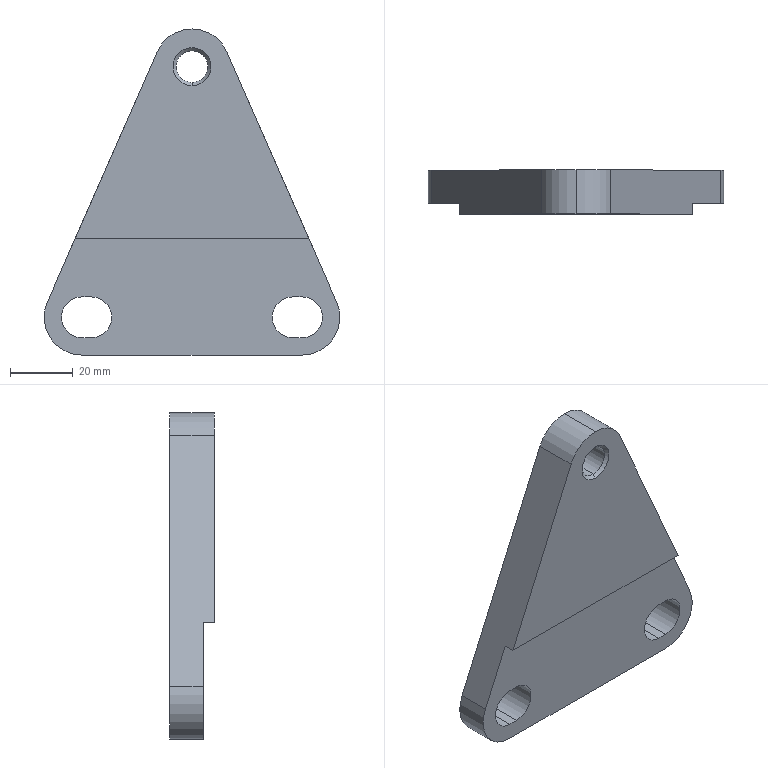Part | SolidWorks | features BaseBody 1 | 1 solid | 25 faces | box 94 x 14 x 103.649 mm | volume 70414 mm3 | plane 11 | cylinder 10 | cone 4 | commonest cylinder face diameters 13 x4 24 x4 10.106 x2
STEP:
#1=CARTESIAN_POINT('',(0.,-13.,96.702));
#2=VERTEX_POINT('',#1);
#3=CARTESIAN_POINT('',(0.,-13.,86.596));
#4=VERTEX_POINT('',#3);
#5=CARTESIAN_POINT('',(0.,-13.,91.649));
#6=DIRECTION('',(0.,-1.,0.));
#7=DIRECTION('',(0.,0.,-1.));
#8=AXIS2_PLACEMENT_3D('',#5,#6,#7);
#9=CIRCLE('',#8,5.053);
#10=EDGE_CURVE('',#2,#4,#9,.T.);
#11=ORIENTED_EDGE('',*,*,#10,.F.);
#12=CARTESIAN_POINT('',(0.,-14.,97.702));
#13=VERTEX_POINT('',#12);
#14=CARTESIAN_POINT('',(0.,-13.,96.702));
#15=DIRECTION('',(0.,-0.7071,0.7071));
#16=VECTOR('',#15,1000.);
#17=LINE('',#14,#16);
#18=EDGE_CURVE('',#2,#13,#17,.T.);
#19=ORIENTED_EDGE('',*,*,#18,.T.);
#20=CARTESIAN_POINT('',(0.,-14.,85.596));
#21=VERTEX_POINT('',#20);
#22=CARTESIAN_POINT('',(0.,-14.,91.649));
#23=DIRECTION('',(0.,1.,0.));
#24=DIRECTION('',(0.,0.,-1.));
#25=AXIS2_PLACEMENT_3D('',#22,#23,#24);
#26=CIRCLE('',#25,6.053);
#27=EDGE_CURVE('',#21,#13,#26,.T.);
#28=ORIENTED_EDGE('',*,*,#27,.F.);
#29=CARTESIAN_POINT('',(0.,-13.,86.596));
#30=DIRECTION('',(0.,-0.7071,-0.7071));
#31=VECTOR('',#30,1000.);
#32=LINE('',#29,#31);
#33=EDGE_CURVE('',#4,#21,#32,.T.);
#34=ORIENTED_EDGE('',*,*,#33,.F.);
#35=EDGE_LOOP('',(#11,#19,#28,#34));
#36=FACE_OUTER_BOUND('',#35,.T.);
#37=CARTESIAN_POINT('',(0.,-13.,91.649));
#38=DIRECTION('',(0.,-1.,0.));
#39=DIRECTION('',(0.,0.,-1.));
#40=AXIS2_PLACEMENT_3D('',#37,#38,#39);
#41=CONICAL_SURFACE('',#40,5.053,0.7854);
#42=ADVANCED_FACE('',(#36),#41,.F.);
#43=CARTESIAN_POINT('',(10.986,0.,96.477));
#44=VERTEX_POINT('',#43);
#45=CARTESIAN_POINT('',(0.,0.,103.649));
#46=VERTEX_POINT('',#45);
#47=CARTESIAN_POINT('',(0.,0.,91.649));
#48=DIRECTION('',(0.,-1.,0.));
#49=DIRECTION('',(1.,0.,0.));
#50=AXIS2_PLACEMENT_3D('',#47,#48,#49);
#51=CIRCLE('',#50,12.);
#52=EDGE_CURVE('',#44,#46,#51,.T.);
#53=ORIENTED_EDGE('',*,*,#52,.T.);
#54=CARTESIAN_POINT('',(0.,-14.,103.649));
#55=VERTEX_POINT('',#54);
#56=CARTESIAN_POINT('',(0.,-14.,103.649));
#57=DIRECTION('',(0.,-1.,0.));
#58=VECTOR('',#57,1000.);
#59=LINE('',#56,#58);
#60=EDGE_CURVE('',#46,#55,#59,.T.);
#61=ORIENTED_EDGE('',*,*,#60,.T.);
#62=CARTESIAN_POINT('',(10.986,-14.,96.477));
#63=VERTEX_POINT('',#62);
#64=CARTESIAN_POINT('',(0.,-14.,91.649));
#65=DIRECTION('',(0.,-1.,0.));
#66=DIRECTION('',(1.,0.,0.));
#67=AXIS2_PLACEMENT_3D('',#64,#65,#66);
#68=CIRCLE('',#67,12.);
#69=EDGE_CURVE('',#63,#55,#68,.T.);
#70=ORIENTED_EDGE('',*,*,#69,.F.);
#71=CARTESIAN_POINT('',(10.986,-14.,96.477));
#72=DIRECTION('',(0.,1.,0.));
#73=VECTOR('',#72,1000.);
#74=LINE('',#71,#73);
#75=EDGE_CURVE('',#63,#44,#74,.T.);
#76=ORIENTED_EDGE('',*,*,#75,.T.);
#77=EDGE_LOOP('',(#53,#61,#70,#76));
#78=FACE_OUTER_BOUND('',#77,.T.);
#79=CARTESIAN_POINT('',(0.,-14.,91.649));
#80=DIRECTION('',(0.,-1.,0.));
#81=DIRECTION('',(0.,0.,1.));
#82=AXIS2_PLACEMENT_3D('',#79,#80,#81);
#83=CYLINDRICAL_SURFACE('',#82,12.);
#84=ADVANCED_FACE('',(#78),#83,.T.);
#85=CARTESIAN_POINT('',(0.,-1.,86.596));
#86=VERTEX_POINT('',#85);
#87=CARTESIAN_POINT('',(0.,-1.,96.702));
#88=VERTEX_POINT('',#87);
#89=CARTESIAN_POINT('',(0.,-1.,91.649));
#90=DIRECTION('',(0.,1.,0.));
#91=DIRECTION('',(0.,0.,-1.));
#92=AXIS2_PLACEMENT_3D('',#89,#90,#91);
#93=CIRCLE('',#92,5.053);
#94=EDGE_CURVE('',#86,#88,#93,.T.);
#95=ORIENTED_EDGE('',*,*,#94,.F.);
#96=CARTESIAN_POINT('',(0.,0.,85.596));
#97=VERTEX_POINT('',#96);
#98=CARTESIAN_POINT('',(0.,0.,85.596));
#99=DIRECTION('',(0.,0.7071,-0.7071));
#100=VECTOR('',#99,1000.);
#101=LINE('',#98,#100);
#102=EDGE_CURVE('',#86,#97,#101,.T.);
#103=ORIENTED_EDGE('',*,*,#102,.T.);
#104=CARTESIAN_POINT('',(0.,0.,97.702));
#105=VERTEX_POINT('',#104);
#106=CARTESIAN_POINT('',(0.,0.,91.649));
#107=DIRECTION('',(0.,-1.,0.));
#108=DIRECTION('',(0.,0.,-1.));
#109=AXIS2_PLACEMENT_3D('',#106,#107,#108);
#110=CIRCLE('',#109,6.053);
#111=EDGE_CURVE('',#105,#97,#110,.T.);
#112=ORIENTED_EDGE('',*,*,#111,.F.);
#113=CARTESIAN_POINT('',(0.,0.,97.702));
#114=DIRECTION('',(0.,0.7071,0.7071));
#115=VECTOR('',#114,1000.);
#116=LINE('',#113,#115);
#117=EDGE_CURVE('',#88,#105,#116,.T.);
#118=ORIENTED_EDGE('',*,*,#117,.F.);
#119=EDGE_LOOP('',(#95,#103,#112,#118));
#120=FACE_OUTER_BOUND('',#119,.T.);
#121=CARTESIAN_POINT('',(0.,0.,91.649));
#122=DIRECTION('',(0.,1.,0.));
#123=DIRECTION('',(0.,0.,1.));
#124=AXIS2_PLACEMENT_3D('',#121,#122,#123);
#125=CONICAL_SURFACE('',#124,6.053,0.7854);
#126=ADVANCED_FACE('',(#120),#125,.F.);
#127=ORIENTED_EDGE('',*,*,#10,.T.);
#128=CARTESIAN_POINT('',(0.,-14.,86.596));
#129=DIRECTION('',(0.,1.,0.));
#130=VECTOR('',#129,1000.);
#131=LINE('',#128,#130);
#132=EDGE_CURVE('',#4,#86,#131,.T.);
#133=ORIENTED_EDGE('',*,*,#132,.T.);
#134=ORIENTED_EDGE('',*,*,#94,.T.);
#135=CARTESIAN_POINT('',(0.,-14.,96.702));
#136=DIRECTION('',(0.,1.,0.));
#137=VECTOR('',#136,1000.);
#138=LINE('',#135,#137);
#139=EDGE_CURVE('',#2,#88,#138,.T.);
#140=ORIENTED_EDGE('',*,*,#139,.F.);
#141=EDGE_LOOP('',(#127,#133,#134,#140));
#142=FACE_OUTER_BOUND('',#141,.T.);
#143=CARTESIAN_POINT('',(0.,-14.,91.649));
#144=DIRECTION('',(0.,1.,0.));
#145=DIRECTION('',(0.,0.,1.));
#146=AXIS2_PLACEMENT_3D('',#143,#144,#145);
#147=CYLINDRICAL_SURFACE('',#146,5.053);
#148=ADVANCED_FACE('',(#142),#147,.F.);
#149=CARTESIAN_POINT('',(-35.,0.,5.5));
#150=VERTEX_POINT('',#149);
#151=CARTESIAN_POINT('',(-35.,-10.5,5.5));
#152=VERTEX_POINT('',#151);
#153=CARTESIAN_POINT('',(-35.,0.,5.5));
#154=DIRECTION('',(0.,-1.,0.));
#155=VECTOR('',#154,1000.);
#156=LINE('',#153,#155);
#157=EDGE_CURVE('',#150,#152,#156,.T.);
#158=ORIENTED_EDGE('',*,*,#157,.T.);
#159=CARTESIAN_POINT('',(-32.,-10.5,5.5));
#160=VERTEX_POINT('',#159);
#161=CARTESIAN_POINT('',(-35.,-10.5,5.5));
#162=DIRECTION('',(1.,0.,0.));
#163=VECTOR('',#162,1000.);
#164=LINE('',#161,#163);
#165=EDGE_CURVE('',#152,#160,#164,.T.);
#166=ORIENTED_EDGE('',*,*,#165,.T.);
#167=CARTESIAN_POINT('',(-32.,0.,5.5));
#168=VERTEX_POINT('',#167);
#169=CARTESIAN_POINT('',(-32.,0.,5.5));
#170=DIRECTION('',(0.,-1.,0.));
#171=VECTOR('',#170,1000.);
#172=LINE('',#169,#171);
#173=EDGE_CURVE('',#168,#160,#172,.T.);
#174=ORIENTED_EDGE('',*,*,#173,.F.);
#175=CARTESIAN_POINT('',(-35.,0.,5.5));
#176=DIRECTION('',(-1.,0.,0.));
#177=VECTOR('',#176,1000.);
#178=LINE('',#175,#177);
#179=EDGE_CURVE('',#168,#150,#178,.T.);
#180=ORIENTED_EDGE('',*,*,#179,.T.);
#181=EDGE_LOOP('',(#158,#166,#174,#180));
#182=FACE_OUTER_BOUND('',#181,.T.);
#183=CARTESIAN_POINT('',(-35.,0.,5.5));
#184=DIRECTION('',(0.,0.,1.));
#185=DIRECTION('',(1.,0.,0.));
#186=AXIS2_PLACEMENT_3D('',#183,#184,#185);
#187=PLANE('',#186);
#188=ADVANCED_FACE('',(#182),#187,.T.);
#189=ORIENTED_EDGE('',*,*,#132,.F.);
#190=CARTESIAN_POINT('',(0.,-13.,91.649));
#191=DIRECTION('',(0.,-1.,0.));
#192=DIRECTION('',(0.,0.,-1.));
#193=AXIS2_PLACEMENT_3D('',#190,#191,#192);
#194=CIRCLE('',#193,5.053);
#195=EDGE_CURVE('',#4,#2,#194,.T.);
#196=ORIENTED_EDGE('',*,*,#195,.T.);
#197=ORIENTED_EDGE('',*,*,#139,.T.);
#198=CARTESIAN_POINT('',(0.,-1.,91.649));
#199=DIRECTION('',(0.,1.,0.));
#200=DIRECTION('',(0.,0.,-1.));
#201=AXIS2_PLACEMENT_3D('',#198,#199,#200);
#202=CIRCLE('',#201,5.053);
#203=EDGE_CURVE('',#88,#86,#202,.T.);
#204=ORIENTED_EDGE('',*,*,#203,.T.);
#205=EDGE_LOOP('',(#189,#196,#197,#204));
#206=FACE_OUTER_BOUND('',#205,.T.);
#207=CARTESIAN_POINT('',(0.,-14.,91.649));
#208=DIRECTION('',(0.,1.,0.));
#209=DIRECTION('',(0.,0.,1.));
#210=AXIS2_PLACEMENT_3D('',#207,#208,#209);
#211=CYLINDRICAL_SURFACE('',#210,5.053);
#212=ADVANCED_FACE('',(#206),#211,.F.);
#213=ORIENTED_EDGE('',*,*,#102,.F.);
#214=ORIENTED_EDGE('',*,*,#203,.F.);
#215=ORIENTED_EDGE('',*,*,#117,.T.);
#216=CARTESIAN_POINT('',(0.,0.,91.649));
#217=DIRECTION('',(0.,-1.,0.));
#218=DIRECTION('',(0.,0.,-1.));
#219=AXIS2_PLACEMENT_3D('',#216,#217,#218);
#220=CIRCLE('',#219,6.053);
#221=EDGE_CURVE('',#97,#105,#220,.T.);
#222=ORIENTED_EDGE('',*,*,#221,.F.);
#223=EDGE_LOOP('',(#213,#214,#215,#222));
#224=FACE_OUTER_BOUND('',#223,.T.);
#225=CARTESIAN_POINT('',(0.,0.,91.649));
#226=DIRECTION('',(0.,1.,0.));
#227=DIRECTION('',(0.,0.,1.));
#228=AXIS2_PLACEMENT_3D('',#225,#226,#227);
#229=CONICAL_SURFACE('',#228,6.053,0.7854);
#230=ADVANCED_FACE('',(#224),#229,.F.);
#231=ORIENTED_EDGE('',*,*,#60,.F.);
#232=CARTESIAN_POINT('',(-10.986,0.,96.477));
#233=VERTEX_POINT('',#232);
#234=CARTESIAN_POINT('',(0.,0.,91.649));
#235=DIRECTION('',(0.,-1.,0.));
#236=DIRECTION('',(1.,0.,0.));
#237=AXIS2_PLACEMENT_3D('',#234,#235,#236);
#238=CIRCLE('',#237,12.);
#239=EDGE_CURVE('',#46,#233,#238,.T.);
#240=ORIENTED_EDGE('',*,*,#239,.T.);
#241=CARTESIAN_POINT('',(-10.986,-14.,96.477));
#242=VERTEX_POINT('',#241);
#243=CARTESIAN_POINT('',(-10.986,-14.,96.477));
#244=DIRECTION('',(0.,1.,0.));
#245=VECTOR('',#244,1000.);
#246=LINE('',#243,#245);
#247=EDGE_CURVE('',#242,#233,#246,.T.);
#248=ORIENTED_EDGE('',*,*,#247,.F.);
#249=CARTESIAN_POINT('',(0.,-14.,91.649));
#250=DIRECTION('',(0.,-1.,0.));
#251=DIRECTION('',(1.,0.,0.));
#252=AXIS2_PLACEMENT_3D('',#249,#250,#251);
#253=CIRCLE('',#252,12.);
#254=EDGE_CURVE('',#55,#242,#253,.T.);
#255=ORIENTED_EDGE('',*,*,#254,.F.);
#256=EDGE_LOOP('',(#231,#240,#248,#255));
#257=FACE_OUTER_BOUND('',#256,.T.);
#258=CARTESIAN_POINT('',(0.,-14.,91.649));
#259=DIRECTION('',(0.,-1.,0.));
#260=DIRECTION('',(0.,0.,1.));
#261=AXIS2_PLACEMENT_3D('',#258,#259,#260);
#262=CYLINDRICAL_SURFACE('',#261,12.);
#263=ADVANCED_FACE('',(#257),#262,.T.);
#264=CARTESIAN_POINT('',(35.,-10.5,0.));
#265=VERTEX_POINT('',#264);
#266=CARTESIAN_POINT('',(45.986,-10.5,16.828));
#267=VERTEX_POINT('',#266);
#268=CARTESIAN_POINT('',(35.,-10.5,12.));
#269=DIRECTION('',(0.,-1.,0.));
#270=DIRECTION('',(0.,0.,-1.));
#271=AXIS2_PLACEMENT_3D('',#268,#269,#270);
#272=CIRCLE('',#271,12.);
#273=EDGE_CURVE('',#265,#267,#272,.T.);
#274=ORIENTED_EDGE('',*,*,#273,.F.);
#275=CARTESIAN_POINT('',(35.,0.,0.));
#276=VERTEX_POINT('',#275);
#277=CARTESIAN_POINT('',(35.,-14.,0.));
#278=DIRECTION('',(0.,1.,0.));
#279=VECTOR('',#278,1000.);
#280=LINE('',#277,#279);
#281=EDGE_CURVE('',#265,#276,#280,.T.);
#282=ORIENTED_EDGE('',*,*,#281,.T.);
#283=CARTESIAN_POINT('',(45.986,0.,16.828));
#284=VERTEX_POINT('',#283);
#285=CARTESIAN_POINT('',(35.,0.,12.));
#286=DIRECTION('',(0.,-1.,0.));
#287=DIRECTION('',(-1.,0.,0.));
#288=AXIS2_PLACEMENT_3D('',#285,#286,#287);
#289=CIRCLE('',#288,12.);
#290=EDGE_CURVE('',#276,#284,#289,.T.);
#291=ORIENTED_EDGE('',*,*,#290,.T.);
#292=CARTESIAN_POINT('',(45.986,-14.,16.828));
#293=DIRECTION('',(0.,1.,0.));
#294=VECTOR('',#293,1000.);
#295=LINE('',#292,#294);
#296=EDGE_CURVE('',#267,#284,#295,.T.);
#297=ORIENTED_EDGE('',*,*,#296,.F.);
#298=EDGE_LOOP('',(#274,#282,#291,#297));
#299=FACE_OUTER_BOUND('',#298,.T.);
#300=CARTESIAN_POINT('',(35.,-14.,12.));
#301=DIRECTION('',(0.,-1.,0.));
#302=DIRECTION('',(0.,0.,1.));
#303=AXIS2_PLACEMENT_3D('',#300,#301,#302);
#304=CYLINDRICAL_SURFACE('',#303,12.);
#305=ADVANCED_FACE('',(#299),#304,.T.);
#306=CARTESIAN_POINT('',(-35.,-10.5,0.));
#307=VERTEX_POINT('',#306);
#308=CARTESIAN_POINT('',(-50.,-10.5,0.));
#309=DIRECTION('',(1.,0.,0.));
#310=VECTOR('',#309,1000.);
#311=LINE('',#308,#310);
#312=EDGE_CURVE('',#307,#265,#311,.T.);
#313=ORIENTED_EDGE('',*,*,#312,.F.);
#314=CARTESIAN_POINT('',(-35.,0.,0.));
#315=VERTEX_POINT('',#314);
#316=CARTESIAN_POINT('',(-35.,-14.,0.));
#317=DIRECTION('',(0.,1.,0.));
#318=VECTOR('',#317,1000.);
#319=LINE('',#316,#318);
#320=EDGE_CURVE('',#307,#315,#319,.T.);
#321=ORIENTED_EDGE('',*,*,#320,.T.);
#322=CARTESIAN_POINT('',(-35.,0.,0.));
#323=DIRECTION('',(1.,0.,0.));
#324=VECTOR('',#323,1000.);
#325=LINE('',#322,#324);
#326=EDGE_CURVE('',#315,#276,#325,.T.);
#327=ORIENTED_EDGE('',*,*,#326,.T.);
#328=ORIENTED_EDGE('',*,*,#281,.F.);
#329=EDGE_LOOP('',(#313,#321,#327,#328));
#330=FACE_OUTER_BOUND('',#329,.T.);
#331=CARTESIAN_POINT('',(-35.,-14.,0.));
#332=DIRECTION('',(0.,0.,1.));
#333=DIRECTION('',(1.,0.,0.));
#334=AXIS2_PLACEMENT_3D('',#331,#332,#333);
#335=PLANE('',#334);
#336=ADVANCED_FACE('',(#330),#335,.F.);
#337=CARTESIAN_POINT('',(-37.122,-10.5,37.));
#338=VERTEX_POINT('',#337);
#339=CARTESIAN_POINT('',(-45.986,-10.5,16.828));
#340=VERTEX_POINT('',#339);
#341=CARTESIAN_POINT('',(-10.986,-10.5,96.477));
#342=DIRECTION('',(-0.4023,0.,-0.9155));
#343=VECTOR('',#342,1000.);
#344=LINE('',#341,#343);
#345=EDGE_CURVE('',#338,#340,#344,.T.);
#346=ORIENTED_EDGE('',*,*,#345,.F.);
#347=CARTESIAN_POINT('',(-37.122,-14.,37.));
#348=VERTEX_POINT('',#347);
#349=CARTESIAN_POINT('',(-37.122,-14.,37.));
#350=DIRECTION('',(0.,-1.,0.));
#351=VECTOR('',#350,1000.);
#352=LINE('',#349,#351);
#353=EDGE_CURVE('',#338,#348,#352,.T.);
#354=ORIENTED_EDGE('',*,*,#353,.T.);
#355=CARTESIAN_POINT('',(-10.986,-14.,96.477));
#356=DIRECTION('',(-0.4023,0.,-0.9155));
#357=VECTOR('',#356,1000.);
#358=LINE('',#355,#357);
#359=EDGE_CURVE('',#242,#348,#358,.T.);
#360=ORIENTED_EDGE('',*,*,#359,.F.);
#361=ORIENTED_EDGE('',*,*,#247,.T.);
#362=CARTESIAN_POINT('',(-45.986,0.,16.828));
#363=VERTEX_POINT('',#362);
#364=CARTESIAN_POINT('',(-10.986,0.,96.477));
#365=DIRECTION('',(-0.4023,0.,-0.9155));
#366=VECTOR('',#365,1000.);
#367=LINE('',#364,#366);
#368=EDGE_CURVE('',#233,#363,#367,.T.);
#369=ORIENTED_EDGE('',*,*,#368,.T.);
#370=CARTESIAN_POINT('',(-45.986,-14.,16.828));
#371=DIRECTION('',(0.,1.,0.));
#372=VECTOR('',#371,1000.);
#373=LINE('',#370,#372);
#374=EDGE_CURVE('',#340,#363,#373,.T.);
#375=ORIENTED_EDGE('',*,*,#374,.F.);
#376=EDGE_LOOP('',(#346,#354,#360,#361,#369,#375));
#377=FACE_OUTER_BOUND('',#376,.T.);
#378=CARTESIAN_POINT('',(-10.986,-14.,96.477));
#379=DIRECTION('',(0.9155,0.,-0.4023));
#380=DIRECTION('',(0.,-1.,0.));
#381=AXIS2_PLACEMENT_3D('',#378,#379,#380);
#382=PLANE('',#381);
#383=ADVANCED_FACE('',(#377),#382,.F.);
#384=CARTESIAN_POINT('',(32.,-10.5,18.5));
#385=VERTEX_POINT('',#384);
#386=CARTESIAN_POINT('',(35.,-10.5,18.5));
#387=VERTEX_POINT('',#386);
#388=CARTESIAN_POINT('',(35.,-10.5,18.5));
#389=DIRECTION('',(1.,0.,0.));
#390=VECTOR('',#389,1000.);
#391=LINE('',#388,#390);
#392=EDGE_CURVE('',#385,#387,#391,.T.);
#393=ORIENTED_EDGE('',*,*,#392,.F.);
#394=CARTESIAN_POINT('',(32.,0.,18.5));
#395=VERTEX_POINT('',#394);
#396=CARTESIAN_POINT('',(32.,0.,18.5));
#397=DIRECTION('',(0.,-1.,0.));
#398=VECTOR('',#397,1000.);
#399=LINE('',#396,#398);
#400=EDGE_CURVE('',#395,#385,#399,.T.);
#401=ORIENTED_EDGE('',*,*,#400,.F.);
#402=CARTESIAN_POINT('',(35.,0.,18.5));
#403=VERTEX_POINT('',#402);
#404=CARTESIAN_POINT('',(35.,0.,18.5));
#405=DIRECTION('',(-1.,0.,0.));
#406=VECTOR('',#405,1000.);
#407=LINE('',#404,#406);
#408=EDGE_CURVE('',#403,#395,#407,.T.);
#409=ORIENTED_EDGE('',*,*,#408,.F.);
#410=CARTESIAN_POINT('',(35.,0.,18.5));
#411=DIRECTION('',(0.,-1.,0.));
#412=VECTOR('',#411,1000.);
#413=LINE('',#410,#412);
#414=EDGE_CURVE('',#403,#387,#413,.T.);
#415=ORIENTED_EDGE('',*,*,#414,.T.);
#416=EDGE_LOOP('',(#393,#401,#409,#415));
#417=FACE_OUTER_BOUND('',#416,.T.);
#418=CARTESIAN_POINT('',(35.,0.,18.5));
#419=DIRECTION('',(0.,0.,1.));
#420=DIRECTION('',(1.,0.,0.));
#421=AXIS2_PLACEMENT_3D('',#418,#419,#420);
#422=PLANE('',#421);
#423=ADVANCED_FACE('',(#417),#422,.F.);
#424=CARTESIAN_POINT('',(35.,-10.5,5.5));
#425=VERTEX_POINT('',#424);
#426=CARTESIAN_POINT('',(35.,-10.5,12.));
#427=DIRECTION('',(0.,1.,0.));
#428=DIRECTION('',(0.,0.,-1.));
#429=AXIS2_PLACEMENT_3D('',#426,#427,#428);
#430=CIRCLE('',#429,6.5);
#431=EDGE_CURVE('',#387,#425,#430,.T.);
#432=ORIENTED_EDGE('',*,*,#431,.F.);
#433=ORIENTED_EDGE('',*,*,#414,.F.);
#434=CARTESIAN_POINT('',(35.,0.,5.5));
#435=VERTEX_POINT('',#434);
#436=CARTESIAN_POINT('',(35.,0.,12.));
#437=DIRECTION('',(0.,-1.,0.));
#438=DIRECTION('',(-1.,0.,0.));
#439=AXIS2_PLACEMENT_3D('',#436,#437,#438);
#440=CIRCLE('',#439,6.5);
#441=EDGE_CURVE('',#435,#403,#440,.T.);
#442=ORIENTED_EDGE('',*,*,#441,.F.);
#443=CARTESIAN_POINT('',(35.,0.,5.5));
#444=DIRECTION('',(0.,-1.,0.));
#445=VECTOR('',#444,1000.);
#446=LINE('',#443,#445);
#447=EDGE_CURVE('',#435,#425,#446,.T.);
#448=ORIENTED_EDGE('',*,*,#447,.T.);
#449=EDGE_LOOP('',(#432,#433,#442,#448));
#450=FACE_OUTER_BOUND('',#449,.T.);
#451=CARTESIAN_POINT('',(35.,0.,12.));
#452=DIRECTION('',(0.,1.,0.));
#453=DIRECTION('',(0.,0.,-1.));
#454=AXIS2_PLACEMENT_3D('',#451,#452,#453);
#455=CYLINDRICAL_SURFACE('',#454,6.5);
#456=ADVANCED_FACE('',(#450),#455,.F.);
#457=ORIENTED_EDGE('',*,*,#173,.T.);
#458=CARTESIAN_POINT('',(-32.,-10.5,18.5));
#459=VERTEX_POINT('',#458);
#460=CARTESIAN_POINT('',(-32.,-10.5,12.));
#461=DIRECTION('',(0.,-1.,0.));
#462=DIRECTION('',(0.,0.,-1.));
#463=AXIS2_PLACEMENT_3D('',#460,#461,#462);
#464=CIRCLE('',#463,6.5);
#465=EDGE_CURVE('',#160,#459,#464,.T.);
#466=ORIENTED_EDGE('',*,*,#465,.T.);
#467=CARTESIAN_POINT('',(-32.,0.,18.5));
#468=VERTEX_POINT('',#467);
#469=CARTESIAN_POINT('',(-32.,0.,18.5));
#470=DIRECTION('',(0.,-1.,0.));
#471=VECTOR('',#470,1000.);
#472=LINE('',#469,#471);
#473=EDGE_CURVE('',#468,#459,#472,.T.);
#474=ORIENTED_EDGE('',*,*,#473,.F.);
#475=CARTESIAN_POINT('',(-32.,0.,12.));
#476=DIRECTION('',(0.,1.,0.));
#477=DIRECTION('',(-1.,0.,0.));
#478=AXIS2_PLACEMENT_3D('',#475,#476,#477);
#479=CIRCLE('',#478,6.5);
#480=EDGE_CURVE('',#468,#168,#479,.T.);
#481=ORIENTED_EDGE('',*,*,#480,.T.);
#482=EDGE_LOOP('',(#457,#466,#474,#481));
#483=FACE_OUTER_BOUND('',#482,.T.);
#484=CARTESIAN_POINT('',(-32.,0.,12.));
#485=DIRECTION('',(0.,1.,0.));
#486=DIRECTION('',(0.,0.,-1.));
#487=AXIS2_PLACEMENT_3D('',#484,#485,#486);
#488=CYLINDRICAL_SURFACE('',#487,6.5);
#489=ADVANCED_FACE('',(#483),#488,.F.);
#490=CARTESIAN_POINT('',(-35.,0.,18.5));
#491=VERTEX_POINT('',#490);
#492=CARTESIAN_POINT('',(-35.,0.,12.));
#493=DIRECTION('',(0.,1.,0.));
#494=DIRECTION('',(1.,0.,0.));
#495=AXIS2_PLACEMENT_3D('',#492,#493,#494);
#496=CIRCLE('',#495,6.5);
#497=EDGE_CURVE('',#150,#491,#496,.T.);
#498=ORIENTED_EDGE('',*,*,#497,.F.);
#499=ORIENTED_EDGE('',*,*,#179,.F.);
#500=ORIENTED_EDGE('',*,*,#480,.F.);
#501=CARTESIAN_POINT('',(-35.,0.,18.5));
#502=DIRECTION('',(1.,0.,0.));
#503=VECTOR('',#502,1000.);
#504=LINE('',#501,#503);
#505=EDGE_CURVE('',#491,#468,#504,.T.);
#506=ORIENTED_EDGE('',*,*,#505,.F.);
#507=EDGE_LOOP('',(#498,#499,#500,#506));
#508=FACE_BOUND('',#507,.T.);
#509=ORIENTED_EDGE('',*,*,#52,.F.);
#510=CARTESIAN_POINT('',(45.986,0.,16.828));
#511=DIRECTION('',(-0.4023,0.,0.9155));
#512=VECTOR('',#511,1000.);
#513=LINE('',#510,#512);
#514=EDGE_CURVE('',#284,#44,#513,.T.);
#515=ORIENTED_EDGE('',*,*,#514,.F.);
#516=ORIENTED_EDGE('',*,*,#290,.F.);
#517=ORIENTED_EDGE('',*,*,#326,.F.);
#518=CARTESIAN_POINT('',(-35.,0.,12.));
#519=DIRECTION('',(0.,-1.,0.));
#520=DIRECTION('',(1.,0.,0.));
#521=AXIS2_PLACEMENT_3D('',#518,#519,#520);
#522=CIRCLE('',#521,12.);
#523=EDGE_CURVE('',#363,#315,#522,.T.);
#524=ORIENTED_EDGE('',*,*,#523,.F.);
#525=ORIENTED_EDGE('',*,*,#368,.F.);
#526=ORIENTED_EDGE('',*,*,#239,.F.);
#527=EDGE_LOOP('',(#509,#515,#516,#517,#524,#525,#526));
#528=FACE_OUTER_BOUND('',#527,.T.);
#529=CARTESIAN_POINT('',(32.,0.,5.5));
#530=VERTEX_POINT('',#529);
#531=CARTESIAN_POINT('',(35.,0.,5.5));
#532=DIRECTION('',(1.,0.,0.));
#533=VECTOR('',#532,1000.);
#534=LINE('',#531,#533);
#535=EDGE_CURVE('',#530,#435,#534,.T.);
#536=ORIENTED_EDGE('',*,*,#535,.T.);
#537=ORIENTED_EDGE('',*,*,#441,.T.);
#538=ORIENTED_EDGE('',*,*,#408,.T.);
#539=CARTESIAN_POINT('',(32.,0.,12.));
#540=DIRECTION('',(0.,-1.,0.));
#541=DIRECTION('',(1.,0.,0.));
#542=AXIS2_PLACEMENT_3D('',#539,#540,#541);
#543=CIRCLE('',#542,6.5);
#544=EDGE_CURVE('',#395,#530,#543,.T.);
#545=ORIENTED_EDGE('',*,*,#544,.T.);
#546=EDGE_LOOP('',(#536,#537,#538,#545));
#547=FACE_BOUND('',#546,.T.);
#548=ORIENTED_EDGE('',*,*,#111,.T.);
#549=ORIENTED_EDGE('',*,*,#221,.T.);
#550=EDGE_LOOP('',(#548,#549));
#551=FACE_BOUND('',#550,.T.);
#552=CARTESIAN_POINT('',(0.,0.,91.649));
#553=DIRECTION('',(0.,-1.,0.));
#554=DIRECTION('',(0.,0.,-1.));
#555=AXIS2_PLACEMENT_3D('',#552,#553,#554);
#556=PLANE('',#555);
#557=ADVANCED_FACE('',(#508,#528,#547,#551),#556,.F.);
#558=ORIENTED_EDGE('',*,*,#473,.T.);
#559=CARTESIAN_POINT('',(-35.,-10.5,18.5));
#560=VERTEX_POINT('',#559);
#561=CARTESIAN_POINT('',(-35.,-10.5,18.5));
#562=DIRECTION('',(-1.,0.,0.));
#563=VECTOR('',#562,1000.);
#564=LINE('',#561,#563);
#565=EDGE_CURVE('',#459,#560,#564,.T.);
#566=ORIENTED_EDGE('',*,*,#565,.T.);
#567=CARTESIAN_POINT('',(-35.,0.,18.5));
#568=DIRECTION('',(0.,-1.,0.));
#569=VECTOR('',#568,1000.);
#570=LINE('',#567,#569);
#571=EDGE_CURVE('',#491,#560,#570,.T.);
#572=ORIENTED_EDGE('',*,*,#571,.F.);
#573=ORIENTED_EDGE('',*,*,#505,.T.);
#574=EDGE_LOOP('',(#558,#566,#572,#573));
#575=FACE_OUTER_BOUND('',#574,.T.);
#576=CARTESIAN_POINT('',(-35.,0.,18.5));
#577=DIRECTION('',(0.,0.,-1.));
#578=DIRECTION('',(0.,-1.,0.));
#579=AXIS2_PLACEMENT_3D('',#576,#577,#578);
#580=PLANE('',#579);
#581=ADVANCED_FACE('',(#575),#580,.T.);
#582=ORIENTED_EDGE('',*,*,#571,.T.);
#583=CARTESIAN_POINT('',(-35.,-10.5,12.));
#584=DIRECTION('',(0.,-1.,0.));
#585=DIRECTION('',(0.,0.,-1.));
#586=AXIS2_PLACEMENT_3D('',#583,#584,#585);
#587=CIRCLE('',#586,6.5);
#588=EDGE_CURVE('',#560,#152,#587,.T.);
#589=ORIENTED_EDGE('',*,*,#588,.T.);
#590=ORIENTED_EDGE('',*,*,#157,.F.);
#591=ORIENTED_EDGE('',*,*,#497,.T.);
#592=EDGE_LOOP('',(#582,#589,#590,#591));
#593=FACE_OUTER_BOUND('',#592,.T.);
#594=CARTESIAN_POINT('',(-35.,0.,12.));
#595=DIRECTION('',(0.,1.,0.));
#596=DIRECTION('',(0.,0.,-1.));
#597=AXIS2_PLACEMENT_3D('',#594,#595,#596);
#598=CYLINDRICAL_SURFACE('',#597,6.5);
#599=ADVANCED_FACE('',(#593),#598,.F.);
#600=CARTESIAN_POINT('',(32.,-10.5,5.5));
#601=VERTEX_POINT('',#600);
#602=CARTESIAN_POINT('',(35.,-10.5,5.5));
#603=DIRECTION('',(-1.,0.,0.));
#604=VECTOR('',#603,1000.);
#605=LINE('',#602,#604);
#606=EDGE_CURVE('',#425,#601,#605,.T.);
#607=ORIENTED_EDGE('',*,*,#606,.F.);
#608=ORIENTED_EDGE('',*,*,#447,.F.);
#609=ORIENTED_EDGE('',*,*,#535,.F.);
#610=CARTESIAN_POINT('',(32.,0.,5.5));
#611=DIRECTION('',(0.,-1.,0.));
#612=VECTOR('',#611,1000.);
#613=LINE('',#610,#612);
#614=EDGE_CURVE('',#530,#601,#613,.T.);
#615=ORIENTED_EDGE('',*,*,#614,.T.);
#616=EDGE_LOOP('',(#607,#608,#609,#615));
#617=FACE_OUTER_BOUND('',#616,.T.);
#618=CARTESIAN_POINT('',(35.,0.,5.5));
#619=DIRECTION('',(0.,0.,-1.));
#620=DIRECTION('',(0.,-1.,0.));
#621=AXIS2_PLACEMENT_3D('',#618,#619,#620);
#622=PLANE('',#621);
#623=ADVANCED_FACE('',(#617),#622,.F.);
#624=CARTESIAN_POINT('',(32.,-10.5,12.));
#625=DIRECTION('',(0.,1.,0.));
#626=DIRECTION('',(0.,0.,-1.));
#627=AXIS2_PLACEMENT_3D('',#624,#625,#626);
#628=CIRCLE('',#627,6.5);
#629=EDGE_CURVE('',#601,#385,#628,.T.);
#630=ORIENTED_EDGE('',*,*,#629,.F.);
#631=ORIENTED_EDGE('',*,*,#614,.F.);
#632=ORIENTED_EDGE('',*,*,#544,.F.);
#633=ORIENTED_EDGE('',*,*,#400,.T.);
#634=EDGE_LOOP('',(#630,#631,#632,#633));
#635=FACE_OUTER_BOUND('',#634,.T.);
#636=CARTESIAN_POINT('',(32.,0.,12.));
#637=DIRECTION('',(0.,1.,0.));
#638=DIRECTION('',(0.,0.,-1.));
#639=AXIS2_PLACEMENT_3D('',#636,#637,#638);
#640=CYLINDRICAL_SURFACE('',#639,6.5);
#641=ADVANCED_FACE('',(#635),#640,.F.);
#642=ORIENTED_EDGE('',*,*,#345,.T.);
#643=CARTESIAN_POINT('',(-35.,-10.5,12.));
#644=DIRECTION('',(0.,-1.,0.));
#645=DIRECTION('',(0.,0.,-1.));
#646=AXIS2_PLACEMENT_3D('',#643,#644,#645);
#647=CIRCLE('',#646,12.);
#648=EDGE_CURVE('',#340,#307,#647,.T.);
#649=ORIENTED_EDGE('',*,*,#648,.T.);
#650=ORIENTED_EDGE('',*,*,#312,.T.);
#651=ORIENTED_EDGE('',*,*,#273,.T.);
#652=CARTESIAN_POINT('',(37.122,-10.5,37.));
#653=VERTEX_POINT('',#652);
#654=CARTESIAN_POINT('',(45.986,-10.5,16.828));
#655=DIRECTION('',(-0.4023,0.,0.9155));
#656=VECTOR('',#655,1000.);
#657=LINE('',#654,#656);
#658=EDGE_CURVE('',#267,#653,#657,.T.);
#659=ORIENTED_EDGE('',*,*,#658,.T.);
#660=CARTESIAN_POINT('',(50.,-10.5,37.));
#661=DIRECTION('',(-1.,0.,0.));
#662=VECTOR('',#661,1000.);
#663=LINE('',#660,#662);
#664=EDGE_CURVE('',#653,#338,#663,.T.);
#665=ORIENTED_EDGE('',*,*,#664,.T.);
#666=EDGE_LOOP('',(#642,#649,#650,#651,#659,#665));
#667=FACE_OUTER_BOUND('',#666,.T.);
#668=ORIENTED_EDGE('',*,*,#431,.T.);
#669=ORIENTED_EDGE('',*,*,#606,.T.);
#670=ORIENTED_EDGE('',*,*,#629,.T.);
#671=ORIENTED_EDGE('',*,*,#392,.T.);
#672=EDGE_LOOP('',(#668,#669,#670,#671));
#673=FACE_BOUND('',#672,.T.);
#674=ORIENTED_EDGE('',*,*,#565,.F.);
#675=ORIENTED_EDGE('',*,*,#465,.F.);
#676=ORIENTED_EDGE('',*,*,#165,.F.);
#677=ORIENTED_EDGE('',*,*,#588,.F.);
#678=EDGE_LOOP('',(#674,#675,#676,#677));
#679=FACE_BOUND('',#678,.T.);
#680=CARTESIAN_POINT('',(50.,-10.5,0.));
#681=DIRECTION('',(0.,-1.,0.));
#682=DIRECTION('',(0.,0.,-1.));
#683=AXIS2_PLACEMENT_3D('',#680,#681,#682);
#684=PLANE('',#683);
#685=ADVANCED_FACE('',(#667,#673,#679),#684,.T.);
#686=CARTESIAN_POINT('',(37.122,-14.,37.));
#687=VERTEX_POINT('',#686);
#688=CARTESIAN_POINT('',(45.986,-14.,16.828));
#689=DIRECTION('',(-0.4023,0.,0.9155));
#690=VECTOR('',#689,1000.);
#691=LINE('',#688,#690);
#692=EDGE_CURVE('',#687,#63,#691,.T.);
#693=ORIENTED_EDGE('',*,*,#692,.F.);
#694=CARTESIAN_POINT('',(37.122,-14.,37.));
#695=DIRECTION('',(0.,1.,0.));
#696=VECTOR('',#695,1000.);
#697=LINE('',#694,#696);
#698=EDGE_CURVE('',#687,#653,#697,.T.);
#699=ORIENTED_EDGE('',*,*,#698,.T.);
#700=ORIENTED_EDGE('',*,*,#658,.F.);
#701=ORIENTED_EDGE('',*,*,#296,.T.);
#702=ORIENTED_EDGE('',*,*,#514,.T.);
#703=ORIENTED_EDGE('',*,*,#75,.F.);
#704=EDGE_LOOP('',(#693,#699,#700,#701,#702,#703));
#705=FACE_OUTER_BOUND('',#704,.T.);
#706=CARTESIAN_POINT('',(45.986,-14.,16.828));
#707=DIRECTION('',(-0.9155,0.,-0.4023));
#708=DIRECTION('',(-0.4023,0.,0.9155));
#709=AXIS2_PLACEMENT_3D('',#706,#707,#708);
#710=PLANE('',#709);
#711=ADVANCED_FACE('',(#705),#710,.F.);
#712=ORIENTED_EDGE('',*,*,#27,.T.);
#713=CARTESIAN_POINT('',(0.,-14.,91.649));
#714=DIRECTION('',(0.,1.,0.));
#715=DIRECTION('',(0.,0.,-1.));
#716=AXIS2_PLACEMENT_3D('',#713,#714,#715);
#717=CIRCLE('',#716,6.053);
#718=EDGE_CURVE('',#13,#21,#717,.T.);
#719=ORIENTED_EDGE('',*,*,#718,.T.);
#720=EDGE_LOOP('',(#712,#719));
#721=FACE_BOUND('',#720,.T.);
#722=CARTESIAN_POINT('',(50.,-14.,37.));
#723=DIRECTION('',(-1.,0.,0.));
#724=VECTOR('',#723,1000.);
#725=LINE('',#722,#724);
#726=EDGE_CURVE('',#687,#348,#725,.T.);
#727=ORIENTED_EDGE('',*,*,#726,.F.);
#728=ORIENTED_EDGE('',*,*,#692,.T.);
#729=ORIENTED_EDGE('',*,*,#69,.T.);
#730=ORIENTED_EDGE('',*,*,#254,.T.);
#731=ORIENTED_EDGE('',*,*,#359,.T.);
#732=EDGE_LOOP('',(#727,#728,#729,#730,#731));
#733=FACE_OUTER_BOUND('',#732,.T.);
#734=CARTESIAN_POINT('',(0.,-14.,91.649));
#735=DIRECTION('',(0.,-1.,0.));
#736=DIRECTION('',(0.,0.,-1.));
#737=AXIS2_PLACEMENT_3D('',#734,#735,#736);
#738=PLANE('',#737);
#739=ADVANCED_FACE('',(#721,#733),#738,.T.);
#740=ORIENTED_EDGE('',*,*,#664,.F.);
#741=ORIENTED_EDGE('',*,*,#698,.F.);
#742=ORIENTED_EDGE('',*,*,#726,.T.);
#743=ORIENTED_EDGE('',*,*,#353,.F.);
#744=EDGE_LOOP('',(#740,#741,#742,#743));
#745=FACE_OUTER_BOUND('',#744,.T.);
#746=CARTESIAN_POINT('',(50.,-10.5,37.));
#747=DIRECTION('',(0.,0.,1.));
#748=DIRECTION('',(1.,0.,0.));
#749=AXIS2_PLACEMENT_3D('',#746,#747,#748);
#750=PLANE('',#749);
#751=ADVANCED_FACE('',(#745),#750,.F.);
#752=ORIENTED_EDGE('',*,*,#18,.F.);
#753=ORIENTED_EDGE('',*,*,#195,.F.);
#754=ORIENTED_EDGE('',*,*,#33,.T.);
#755=ORIENTED_EDGE('',*,*,#718,.F.);
#756=EDGE_LOOP('',(#752,#753,#754,#755));
#757=FACE_OUTER_BOUND('',#756,.T.);
#758=CARTESIAN_POINT('',(0.,-13.,91.649));
#759=DIRECTION('',(0.,-1.,0.));
#760=DIRECTION('',(0.,0.,-1.));
#761=AXIS2_PLACEMENT_3D('',#758,#759,#760);
#762=CONICAL_SURFACE('',#761,5.053,0.7854);
#763=ADVANCED_FACE('',(#757),#762,.F.);
#764=ORIENTED_EDGE('',*,*,#648,.F.);
#765=ORIENTED_EDGE('',*,*,#374,.T.);
#766=ORIENTED_EDGE('',*,*,#523,.T.);
#767=ORIENTED_EDGE('',*,*,#320,.F.);
#768=EDGE_LOOP('',(#764,#765,#766,#767));
#769=FACE_OUTER_BOUND('',#768,.T.);
#770=CARTESIAN_POINT('',(-35.,-14.,12.));
#771=DIRECTION('',(0.,-1.,0.));
#772=DIRECTION('',(0.,0.,1.));
#773=AXIS2_PLACEMENT_3D('',#770,#771,#772);
#774=CYLINDRICAL_SURFACE('',#773,12.);
#775=ADVANCED_FACE('',(#769),#774,.T.);
#776=CLOSED_SHELL('',(#42,#84,#126,#148,#188,#212,#230,#263,#305,#336,#383,#423,#456,#489,#557,#581,#599,#623,#641,#685,#711,#739,#751,#763,#775));
#777=MANIFOLD_SOLID_BREP('',#776);
#778=CARTESIAN_POINT('',(0.,0.,0.));
#779=DIRECTION('',(0.,0.,1.));
#780=DIRECTION('',(1.,0.,0.));
#781=AXIS2_PLACEMENT_3D('',#778,#779,#780);
#782=(LENGTH_UNIT()NAMED_UNIT(*)SI_UNIT(.MILLI.,.METRE.));
#783=UNCERTAINTY_MEASURE_WITH_UNIT(LENGTH_MEASURE(0.00001),#782,'','');
#784=(NAMED_UNIT(*)PLANE_ANGLE_UNIT()SI_UNIT($,.RADIAN.));
#785=(NAMED_UNIT(*)SI_UNIT($,.STERADIAN.)SOLID_ANGLE_UNIT());
#786=(GEOMETRIC_REPRESENTATION_CONTEXT(3)GLOBAL_UNCERTAINTY_ASSIGNED_CONTEXT((#783))GLOBAL_UNIT_ASSIGNED_CONTEXT((#782,#784,#785))REPRESENTATION_CONTEXT('',''));
#787=ADVANCED_BREP_SHAPE_REPRESENTATION('',(#777,#781),#786);